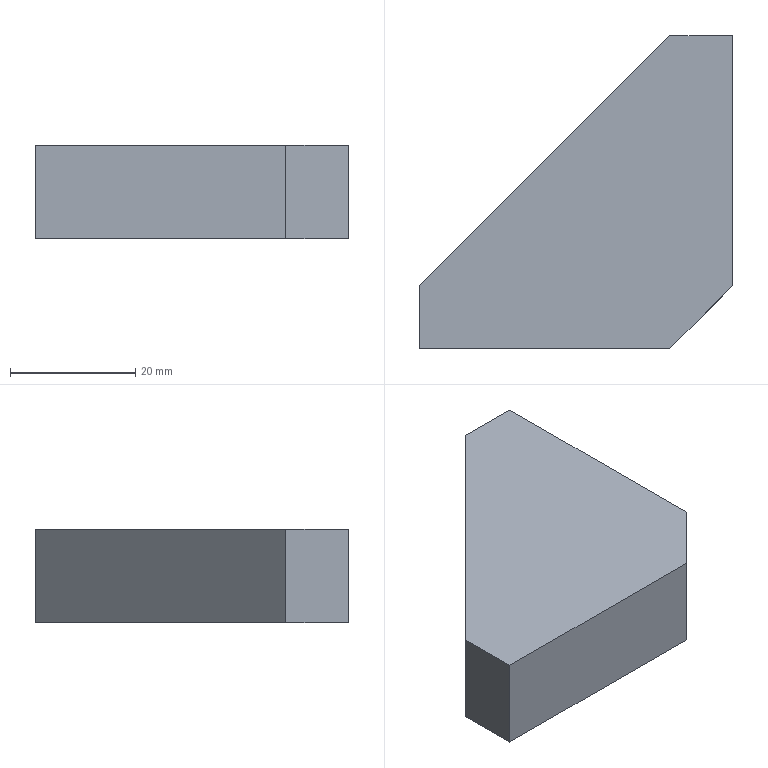Part | SolidWorks | features Extrusion 1 | 1 solid | 8 faces | box 50 x 50 x 15 mm | volume 24750 mm3 | plane 8
STEP:
#1=CARTESIAN_POINT('',(0.,0.,-7.5));
#2=VERTEX_POINT('',#1);
#3=CARTESIAN_POINT('',(40.,0.,-7.5));
#4=VERTEX_POINT('',#3);
#5=CARTESIAN_POINT('',(40.,0.,-7.5));
#6=DIRECTION('',(1.,0.,0.));
#7=VECTOR('',#6,1000.);
#8=LINE('',#5,#7);
#9=EDGE_CURVE('',#2,#4,#8,.T.);
#10=ORIENTED_EDGE('',*,*,#9,.T.);
#11=CARTESIAN_POINT('',(40.,0.,7.5));
#12=VERTEX_POINT('',#11);
#13=CARTESIAN_POINT('',(40.,0.,7.5));
#14=DIRECTION('',(0.,0.,-1.));
#15=VECTOR('',#14,1000.);
#16=LINE('',#13,#15);
#17=EDGE_CURVE('',#12,#4,#16,.T.);
#18=ORIENTED_EDGE('',*,*,#17,.F.);
#19=CARTESIAN_POINT('',(0.,0.,7.5));
#20=VERTEX_POINT('',#19);
#21=CARTESIAN_POINT('',(40.,0.,7.5));
#22=DIRECTION('',(1.,0.,0.));
#23=VECTOR('',#22,1000.);
#24=LINE('',#21,#23);
#25=EDGE_CURVE('',#20,#12,#24,.T.);
#26=ORIENTED_EDGE('',*,*,#25,.F.);
#27=CARTESIAN_POINT('',(0.,0.,7.5));
#28=DIRECTION('',(0.,0.,-1.));
#29=VECTOR('',#28,1000.);
#30=LINE('',#27,#29);
#31=EDGE_CURVE('',#20,#2,#30,.T.);
#32=ORIENTED_EDGE('',*,*,#31,.T.);
#33=EDGE_LOOP('',(#10,#18,#26,#32));
#34=FACE_OUTER_BOUND('',#33,.T.);
#35=CARTESIAN_POINT('',(40.,0.,7.5));
#36=DIRECTION('',(0.,1.,0.));
#37=DIRECTION('',(-1.,0.,0.));
#38=AXIS2_PLACEMENT_3D('',#35,#36,#37);
#39=PLANE('',#38);
#40=ADVANCED_FACE('',(#34),#39,.F.);
#41=CARTESIAN_POINT('',(50.,10.,-7.5));
#42=VERTEX_POINT('',#41);
#43=CARTESIAN_POINT('',(50.,10.,-7.5));
#44=DIRECTION('',(0.7071,0.7071,0.));
#45=VECTOR('',#44,1000.);
#46=LINE('',#43,#45);
#47=EDGE_CURVE('',#4,#42,#46,.T.);
#48=ORIENTED_EDGE('',*,*,#47,.T.);
#49=CARTESIAN_POINT('',(50.,10.,7.5));
#50=VERTEX_POINT('',#49);
#51=CARTESIAN_POINT('',(50.,10.,7.5));
#52=DIRECTION('',(0.,0.,-1.));
#53=VECTOR('',#52,1000.);
#54=LINE('',#51,#53);
#55=EDGE_CURVE('',#50,#42,#54,.T.);
#56=ORIENTED_EDGE('',*,*,#55,.F.);
#57=CARTESIAN_POINT('',(50.,10.,7.5));
#58=DIRECTION('',(0.7071,0.7071,0.));
#59=VECTOR('',#58,1000.);
#60=LINE('',#57,#59);
#61=EDGE_CURVE('',#12,#50,#60,.T.);
#62=ORIENTED_EDGE('',*,*,#61,.F.);
#63=ORIENTED_EDGE('',*,*,#17,.T.);
#64=EDGE_LOOP('',(#48,#56,#62,#63));
#65=FACE_OUTER_BOUND('',#64,.T.);
#66=CARTESIAN_POINT('',(50.,10.,7.5));
#67=DIRECTION('',(-0.7071,0.7071,0.));
#68=DIRECTION('',(-0.7071,-0.7071,0.));
#69=AXIS2_PLACEMENT_3D('',#66,#67,#68);
#70=PLANE('',#69);
#71=ADVANCED_FACE('',(#65),#70,.F.);
#72=CARTESIAN_POINT('',(50.,50.,-7.5));
#73=VERTEX_POINT('',#72);
#74=CARTESIAN_POINT('',(50.,50.,-7.5));
#75=DIRECTION('',(0.,1.,0.));
#76=VECTOR('',#75,1000.);
#77=LINE('',#74,#76);
#78=EDGE_CURVE('',#42,#73,#77,.T.);
#79=ORIENTED_EDGE('',*,*,#78,.T.);
#80=CARTESIAN_POINT('',(50.,50.,7.5));
#81=VERTEX_POINT('',#80);
#82=CARTESIAN_POINT('',(50.,50.,7.5));
#83=DIRECTION('',(0.,0.,-1.));
#84=VECTOR('',#83,1000.);
#85=LINE('',#82,#84);
#86=EDGE_CURVE('',#81,#73,#85,.T.);
#87=ORIENTED_EDGE('',*,*,#86,.F.);
#88=CARTESIAN_POINT('',(50.,50.,7.5));
#89=DIRECTION('',(0.,1.,0.));
#90=VECTOR('',#89,1000.);
#91=LINE('',#88,#90);
#92=EDGE_CURVE('',#50,#81,#91,.T.);
#93=ORIENTED_EDGE('',*,*,#92,.F.);
#94=ORIENTED_EDGE('',*,*,#55,.T.);
#95=EDGE_LOOP('',(#79,#87,#93,#94));
#96=FACE_OUTER_BOUND('',#95,.T.);
#97=CARTESIAN_POINT('',(50.,50.,7.5));
#98=DIRECTION('',(-1.,0.,0.));
#99=DIRECTION('',(0.,-1.,0.));
#100=AXIS2_PLACEMENT_3D('',#97,#98,#99);
#101=PLANE('',#100);
#102=ADVANCED_FACE('',(#96),#101,.F.);
#103=CARTESIAN_POINT('',(40.,50.,-7.5));
#104=VERTEX_POINT('',#103);
#105=CARTESIAN_POINT('',(40.,50.,-7.5));
#106=DIRECTION('',(-1.,0.,0.));
#107=VECTOR('',#106,1000.);
#108=LINE('',#105,#107);
#109=EDGE_CURVE('',#73,#104,#108,.T.);
#110=ORIENTED_EDGE('',*,*,#109,.T.);
#111=CARTESIAN_POINT('',(40.,50.,7.5));
#112=VERTEX_POINT('',#111);
#113=CARTESIAN_POINT('',(40.,50.,7.5));
#114=DIRECTION('',(0.,0.,-1.));
#115=VECTOR('',#114,1000.);
#116=LINE('',#113,#115);
#117=EDGE_CURVE('',#112,#104,#116,.T.);
#118=ORIENTED_EDGE('',*,*,#117,.F.);
#119=CARTESIAN_POINT('',(40.,50.,7.5));
#120=DIRECTION('',(-1.,0.,0.));
#121=VECTOR('',#120,1000.);
#122=LINE('',#119,#121);
#123=EDGE_CURVE('',#81,#112,#122,.T.);
#124=ORIENTED_EDGE('',*,*,#123,.F.);
#125=ORIENTED_EDGE('',*,*,#86,.T.);
#126=EDGE_LOOP('',(#110,#118,#124,#125));
#127=FACE_OUTER_BOUND('',#126,.T.);
#128=CARTESIAN_POINT('',(40.,50.,7.5));
#129=DIRECTION('',(0.,-1.,0.));
#130=DIRECTION('',(0.,0.,-1.));
#131=AXIS2_PLACEMENT_3D('',#128,#129,#130);
#132=PLANE('',#131);
#133=ADVANCED_FACE('',(#127),#132,.F.);
#134=CARTESIAN_POINT('',(0.,10.,-7.5));
#135=VERTEX_POINT('',#134);
#136=CARTESIAN_POINT('',(0.,10.,-7.5));
#137=DIRECTION('',(-0.7071,-0.7071,0.));
#138=VECTOR('',#137,1000.);
#139=LINE('',#136,#138);
#140=EDGE_CURVE('',#104,#135,#139,.T.);
#141=ORIENTED_EDGE('',*,*,#140,.T.);
#142=CARTESIAN_POINT('',(0.,10.,7.5));
#143=VERTEX_POINT('',#142);
#144=CARTESIAN_POINT('',(0.,10.,7.5));
#145=DIRECTION('',(0.,0.,-1.));
#146=VECTOR('',#145,1000.);
#147=LINE('',#144,#146);
#148=EDGE_CURVE('',#143,#135,#147,.T.);
#149=ORIENTED_EDGE('',*,*,#148,.F.);
#150=CARTESIAN_POINT('',(0.,10.,7.5));
#151=DIRECTION('',(-0.7071,-0.7071,0.));
#152=VECTOR('',#151,1000.);
#153=LINE('',#150,#152);
#154=EDGE_CURVE('',#112,#143,#153,.T.);
#155=ORIENTED_EDGE('',*,*,#154,.F.);
#156=ORIENTED_EDGE('',*,*,#117,.T.);
#157=EDGE_LOOP('',(#141,#149,#155,#156));
#158=FACE_OUTER_BOUND('',#157,.T.);
#159=CARTESIAN_POINT('',(0.,10.,7.5));
#160=DIRECTION('',(0.7071,-0.7071,0.));
#161=DIRECTION('',(0.7071,0.7071,0.));
#162=AXIS2_PLACEMENT_3D('',#159,#160,#161);
#163=PLANE('',#162);
#164=ADVANCED_FACE('',(#158),#163,.F.);
#165=CARTESIAN_POINT('',(0.,0.,-7.5));
#166=DIRECTION('',(0.,-1.,0.));
#167=VECTOR('',#166,1000.);
#168=LINE('',#165,#167);
#169=EDGE_CURVE('',#135,#2,#168,.T.);
#170=ORIENTED_EDGE('',*,*,#169,.T.);
#171=ORIENTED_EDGE('',*,*,#31,.F.);
#172=CARTESIAN_POINT('',(0.,0.,7.5));
#173=DIRECTION('',(0.,-1.,0.));
#174=VECTOR('',#173,1000.);
#175=LINE('',#172,#174);
#176=EDGE_CURVE('',#143,#20,#175,.T.);
#177=ORIENTED_EDGE('',*,*,#176,.F.);
#178=ORIENTED_EDGE('',*,*,#148,.T.);
#179=EDGE_LOOP('',(#170,#171,#177,#178));
#180=FACE_OUTER_BOUND('',#179,.T.);
#181=CARTESIAN_POINT('',(0.,0.,7.5));
#182=DIRECTION('',(1.,0.,0.));
#183=DIRECTION('',(0.,0.,-1.));
#184=AXIS2_PLACEMENT_3D('',#181,#182,#183);
#185=PLANE('',#184);
#186=ADVANCED_FACE('',(#180),#185,.F.);
#187=ORIENTED_EDGE('',*,*,#25,.T.);
#188=ORIENTED_EDGE('',*,*,#61,.T.);
#189=ORIENTED_EDGE('',*,*,#92,.T.);
#190=ORIENTED_EDGE('',*,*,#123,.T.);
#191=ORIENTED_EDGE('',*,*,#154,.T.);
#192=ORIENTED_EDGE('',*,*,#176,.T.);
#193=EDGE_LOOP('',(#187,#188,#189,#190,#191,#192));
#194=FACE_OUTER_BOUND('',#193,.T.);
#195=CARTESIAN_POINT('',(0.,0.,7.5));
#196=DIRECTION('',(0.,0.,-1.));
#197=DIRECTION('',(-1.,0.,0.));
#198=AXIS2_PLACEMENT_3D('',#195,#196,#197);
#199=PLANE('',#198);
#200=ADVANCED_FACE('',(#194),#199,.F.);
#201=ORIENTED_EDGE('',*,*,#9,.F.);
#202=ORIENTED_EDGE('',*,*,#169,.F.);
#203=ORIENTED_EDGE('',*,*,#140,.F.);
#204=ORIENTED_EDGE('',*,*,#109,.F.);
#205=ORIENTED_EDGE('',*,*,#78,.F.);
#206=ORIENTED_EDGE('',*,*,#47,.F.);
#207=EDGE_LOOP('',(#201,#202,#203,#204,#205,#206));
#208=FACE_OUTER_BOUND('',#207,.T.);
#209=CARTESIAN_POINT('',(0.,0.,-7.5));
#210=DIRECTION('',(0.,0.,-1.));
#211=DIRECTION('',(-1.,0.,0.));
#212=AXIS2_PLACEMENT_3D('',#209,#210,#211);
#213=PLANE('',#212);
#214=ADVANCED_FACE('',(#208),#213,.T.);
#215=CLOSED_SHELL('',(#40,#71,#102,#133,#164,#186,#200,#214));
#216=MANIFOLD_SOLID_BREP('',#215);
#217=CARTESIAN_POINT('',(0.,0.,0.));
#218=DIRECTION('',(0.,0.,1.));
#219=DIRECTION('',(1.,0.,0.));
#220=AXIS2_PLACEMENT_3D('',#217,#218,#219);
#221=(LENGTH_UNIT()NAMED_UNIT(*)SI_UNIT(.MILLI.,.METRE.));
#222=UNCERTAINTY_MEASURE_WITH_UNIT(LENGTH_MEASURE(0.00001),#221,'','');
#223=(NAMED_UNIT(*)PLANE_ANGLE_UNIT()SI_UNIT($,.RADIAN.));
#224=(NAMED_UNIT(*)SI_UNIT($,.STERADIAN.)SOLID_ANGLE_UNIT());
#225=(GEOMETRIC_REPRESENTATION_CONTEXT(3)GLOBAL_UNCERTAINTY_ASSIGNED_CONTEXT((#222))GLOBAL_UNIT_ASSIGNED_CONTEXT((#221,#223,#224))REPRESENTATION_CONTEXT('',''));
#226=ADVANCED_BREP_SHAPE_REPRESENTATION('',(#216,#220),#225);